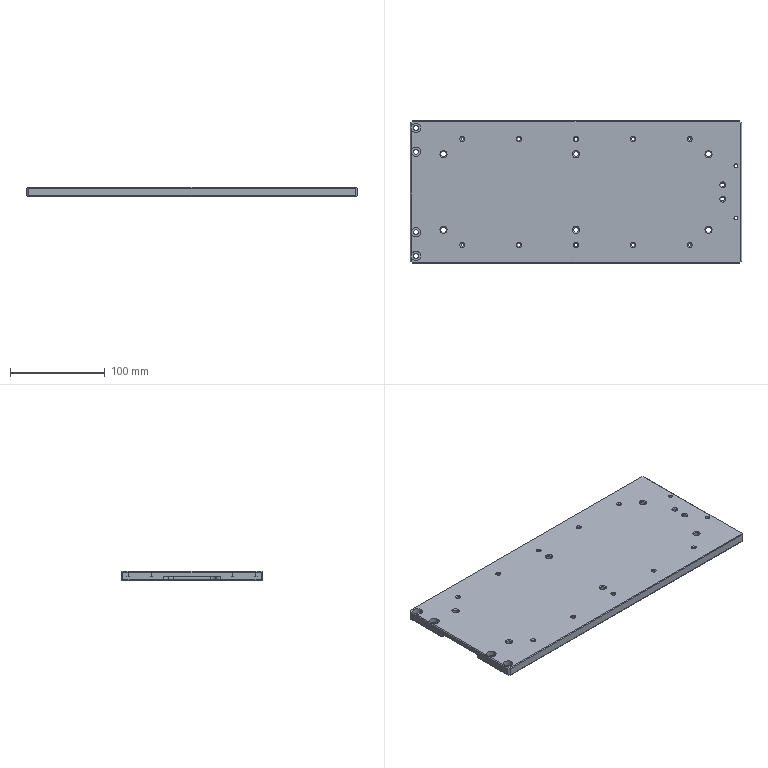Part | STEP file | 1 solid | 216 faces | box 350 x 150 x 10 mm | volume 449712 mm3 | cone 88 | cylinder 84 | plane 44 | commonest cylinder face diameters 10 x24 3.3 x20 5.5 x20 4 x12 4.2 x8